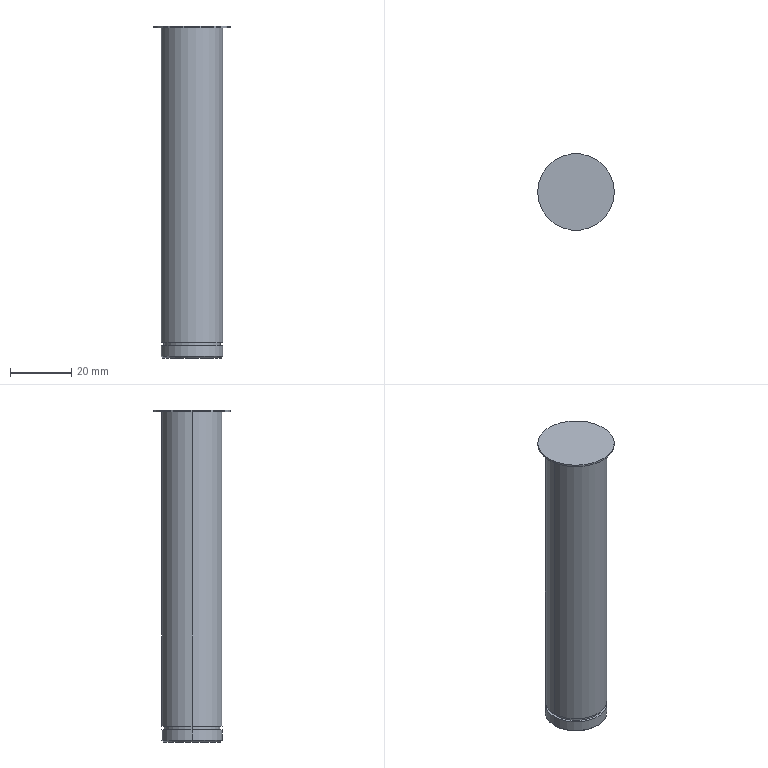Part | SolidWorks | features BaseBody 1 | 1 solid | 15 faces | box 25 x 25 x 108.34 mm | volume 34075 mm3 | cylinder 8 | plane 5 | cone 2 | commonest cylinder face diameters 20 x4 18.35 x2 25 x2
STEP:
#1=CARTESIAN_POINT('',(-9.5,0.,0.));
#2=VERTEX_POINT('',#1);
#3=CARTESIAN_POINT('',(9.5,0.,0.));
#4=VERTEX_POINT('',#3);
#5=CARTESIAN_POINT('',(0.,0.,0.));
#6=DIRECTION('',(0.,0.,1.));
#7=DIRECTION('',(-1.,0.,0.));
#8=AXIS2_PLACEMENT_3D('',#5,#6,#7);
#9=CIRCLE('',#8,9.5);
#10=EDGE_CURVE('',#2,#4,#9,.T.);
#11=ORIENTED_EDGE('',*,*,#10,.T.);
#12=CARTESIAN_POINT('',(10.,0.,0.5));
#13=VERTEX_POINT('',#12);
#14=CARTESIAN_POINT('',(9.75,0.,0.25));
#15=DIRECTION('',(0.7071,0.,0.7071));
#16=VECTOR('',#15,1000.);
#17=LINE('',#14,#16);
#18=EDGE_CURVE('',#4,#13,#17,.T.);
#19=ORIENTED_EDGE('',*,*,#18,.T.);
#20=CARTESIAN_POINT('',(-10.,0.,0.5));
#21=VERTEX_POINT('',#20);
#22=CARTESIAN_POINT('',(0.,0.,0.5));
#23=DIRECTION('',(0.,0.,-1.));
#24=DIRECTION('',(-1.,0.,0.));
#25=AXIS2_PLACEMENT_3D('',#22,#23,#24);
#26=CIRCLE('',#25,10.);
#27=EDGE_CURVE('',#13,#21,#26,.T.);
#28=ORIENTED_EDGE('',*,*,#27,.T.);
#29=CARTESIAN_POINT('',(-9.75,0.,0.25));
#30=DIRECTION('',(-0.7071,0.,0.7071));
#31=VECTOR('',#30,1000.);
#32=LINE('',#29,#31);
#33=EDGE_CURVE('',#2,#21,#32,.T.);
#34=ORIENTED_EDGE('',*,*,#33,.F.);
#35=EDGE_LOOP('',(#11,#19,#28,#34));
#36=FACE_OUTER_BOUND('',#35,.T.);
#37=CARTESIAN_POINT('',(0.,0.,0.25));
#38=DIRECTION('',(0.,0.,1.));
#39=DIRECTION('',(-1.,0.,0.));
#40=AXIS2_PLACEMENT_3D('',#37,#38,#39);
#41=CONICAL_SURFACE('',#40,9.75,0.7854);
#42=ADVANCED_FACE('',(#36),#41,.T.);
#43=CARTESIAN_POINT('',(-10.,0.,4.));
#44=VERTEX_POINT('',#43);
#45=CARTESIAN_POINT('',(10.,0.,4.));
#46=VERTEX_POINT('',#45);
#47=CARTESIAN_POINT('',(0.,0.,4.));
#48=DIRECTION('',(0.,0.,-1.));
#49=DIRECTION('',(-1.,0.,0.));
#50=AXIS2_PLACEMENT_3D('',#47,#48,#49);
#51=CIRCLE('',#50,10.);
#52=EDGE_CURVE('',#44,#46,#51,.T.);
#53=ORIENTED_EDGE('',*,*,#52,.T.);
#54=CARTESIAN_POINT('',(10.,0.,0.));
#55=DIRECTION('',(0.,0.,-1.));
#56=VECTOR('',#55,1000.);
#57=LINE('',#54,#56);
#58=EDGE_CURVE('',#46,#13,#57,.T.);
#59=ORIENTED_EDGE('',*,*,#58,.T.);
#60=CARTESIAN_POINT('',(0.,0.,0.5));
#61=DIRECTION('',(0.,0.,-1.));
#62=DIRECTION('',(-1.,0.,0.));
#63=AXIS2_PLACEMENT_3D('',#60,#61,#62);
#64=CIRCLE('',#63,10.);
#65=EDGE_CURVE('',#21,#13,#64,.T.);
#66=ORIENTED_EDGE('',*,*,#65,.F.);
#67=CARTESIAN_POINT('',(-10.,0.,0.));
#68=DIRECTION('',(0.,0.,-1.));
#69=VECTOR('',#68,1000.);
#70=LINE('',#67,#69);
#71=EDGE_CURVE('',#44,#21,#70,.T.);
#72=ORIENTED_EDGE('',*,*,#71,.F.);
#73=EDGE_LOOP('',(#53,#59,#66,#72));
#74=FACE_OUTER_BOUND('',#73,.T.);
#75=CARTESIAN_POINT('',(0.,0.,0.));
#76=DIRECTION('',(0.,0.,-1.));
#77=DIRECTION('',(-1.,0.,0.));
#78=AXIS2_PLACEMENT_3D('',#75,#76,#77);
#79=CYLINDRICAL_SURFACE('',#78,10.);
#80=ADVANCED_FACE('',(#74),#79,.T.);
#81=CARTESIAN_POINT('',(9.175,0.,5.2));
#82=VERTEX_POINT('',#81);
#83=CARTESIAN_POINT('',(-9.175,0.,5.2));
#84=VERTEX_POINT('',#83);
#85=CARTESIAN_POINT('',(0.,0.,5.2));
#86=DIRECTION('',(0.,0.,1.));
#87=DIRECTION('',(1.,0.,0.));
#88=AXIS2_PLACEMENT_3D('',#85,#86,#87);
#89=CIRCLE('',#88,9.175);
#90=EDGE_CURVE('',#82,#84,#89,.T.);
#91=ORIENTED_EDGE('',*,*,#90,.F.);
#92=CARTESIAN_POINT('',(9.175,0.,4.));
#93=VERTEX_POINT('',#92);
#94=CARTESIAN_POINT('',(9.175,0.,4.6));
#95=DIRECTION('',(0.,0.,-1.));
#96=VECTOR('',#95,1000.);
#97=LINE('',#94,#96);
#98=EDGE_CURVE('',#82,#93,#97,.T.);
#99=ORIENTED_EDGE('',*,*,#98,.T.);
#100=CARTESIAN_POINT('',(-9.175,0.,4.));
#101=VERTEX_POINT('',#100);
#102=CARTESIAN_POINT('',(0.,0.,4.));
#103=DIRECTION('',(0.,0.,1.));
#104=DIRECTION('',(1.,0.,0.));
#105=AXIS2_PLACEMENT_3D('',#102,#103,#104);
#106=CIRCLE('',#105,9.175);
#107=EDGE_CURVE('',#93,#101,#106,.T.);
#108=ORIENTED_EDGE('',*,*,#107,.T.);
#109=CARTESIAN_POINT('',(-9.175,0.,4.6));
#110=DIRECTION('',(0.,0.,-1.));
#111=VECTOR('',#110,1000.);
#112=LINE('',#109,#111);
#113=EDGE_CURVE('',#84,#101,#112,.T.);
#114=ORIENTED_EDGE('',*,*,#113,.F.);
#115=EDGE_LOOP('',(#91,#99,#108,#114));
#116=FACE_OUTER_BOUND('',#115,.T.);
#117=CARTESIAN_POINT('',(0.,0.,4.6));
#118=DIRECTION('',(0.,0.,-1.));
#119=DIRECTION('',(-1.,0.,0.));
#120=AXIS2_PLACEMENT_3D('',#117,#118,#119);
#121=CYLINDRICAL_SURFACE('',#120,9.175);
#122=ADVANCED_FACE('',(#116),#121,.T.);
#123=CARTESIAN_POINT('',(12.5,0.,107.74));
#124=VERTEX_POINT('',#123);
#125=CARTESIAN_POINT('',(-12.5,0.,107.74));
#126=VERTEX_POINT('',#125);
#127=CARTESIAN_POINT('',(0.,0.,107.74));
#128=DIRECTION('',(0.,0.,-1.));
#129=DIRECTION('',(-1.,0.,0.));
#130=AXIS2_PLACEMENT_3D('',#127,#128,#129);
#131=CIRCLE('',#130,12.5);
#132=EDGE_CURVE('',#124,#126,#131,.T.);
#133=ORIENTED_EDGE('',*,*,#132,.F.);
#134=CARTESIAN_POINT('',(12.5,0.,108.34));
#135=VERTEX_POINT('',#134);
#136=CARTESIAN_POINT('',(12.5,0.,108.34));
#137=DIRECTION('',(0.,0.,1.));
#138=VECTOR('',#137,1000.);
#139=LINE('',#136,#138);
#140=EDGE_CURVE('',#124,#135,#139,.T.);
#141=ORIENTED_EDGE('',*,*,#140,.T.);
#142=CARTESIAN_POINT('',(-12.5,0.,108.34));
#143=VERTEX_POINT('',#142);
#144=CARTESIAN_POINT('',(0.,0.,108.34));
#145=DIRECTION('',(0.,0.,-1.));
#146=DIRECTION('',(-1.,0.,0.));
#147=AXIS2_PLACEMENT_3D('',#144,#145,#146);
#148=CIRCLE('',#147,12.5);
#149=EDGE_CURVE('',#135,#143,#148,.T.);
#150=ORIENTED_EDGE('',*,*,#149,.T.);
#151=CARTESIAN_POINT('',(-12.5,0.,108.34));
#152=DIRECTION('',(0.,0.,1.));
#153=VECTOR('',#152,1000.);
#154=LINE('',#151,#153);
#155=EDGE_CURVE('',#126,#143,#154,.T.);
#156=ORIENTED_EDGE('',*,*,#155,.F.);
#157=EDGE_LOOP('',(#133,#141,#150,#156));
#158=FACE_OUTER_BOUND('',#157,.T.);
#159=CARTESIAN_POINT('',(0.,0.,108.34));
#160=DIRECTION('',(0.,0.,1.));
#161=DIRECTION('',(-1.,0.,0.));
#162=AXIS2_PLACEMENT_3D('',#159,#160,#161);
#163=CYLINDRICAL_SURFACE('',#162,12.5);
#164=ADVANCED_FACE('',(#158),#163,.T.);
#165=CARTESIAN_POINT('',(-10.,0.,107.74));
#166=VERTEX_POINT('',#165);
#167=CARTESIAN_POINT('',(10.,0.,107.74));
#168=VERTEX_POINT('',#167);
#169=CARTESIAN_POINT('',(0.,0.,107.74));
#170=DIRECTION('',(0.,0.,-1.));
#171=DIRECTION('',(-1.,0.,0.));
#172=AXIS2_PLACEMENT_3D('',#169,#170,#171);
#173=CIRCLE('',#172,10.);
#174=EDGE_CURVE('',#166,#168,#173,.T.);
#175=ORIENTED_EDGE('',*,*,#174,.T.);
#176=CARTESIAN_POINT('',(10.,0.,5.2));
#177=VERTEX_POINT('',#176);
#178=CARTESIAN_POINT('',(10.,0.,0.));
#179=DIRECTION('',(0.,0.,-1.));
#180=VECTOR('',#179,1000.);
#181=LINE('',#178,#180);
#182=EDGE_CURVE('',#168,#177,#181,.T.);
#183=ORIENTED_EDGE('',*,*,#182,.T.);
#184=CARTESIAN_POINT('',(-10.,0.,5.2));
#185=VERTEX_POINT('',#184);
#186=CARTESIAN_POINT('',(0.,0.,5.2));
#187=DIRECTION('',(0.,0.,1.));
#188=DIRECTION('',(-1.,0.,0.));
#189=AXIS2_PLACEMENT_3D('',#186,#187,#188);
#190=CIRCLE('',#189,10.);
#191=EDGE_CURVE('',#177,#185,#190,.T.);
#192=ORIENTED_EDGE('',*,*,#191,.T.);
#193=CARTESIAN_POINT('',(-10.,0.,0.));
#194=DIRECTION('',(0.,0.,-1.));
#195=VECTOR('',#194,1000.);
#196=LINE('',#193,#195);
#197=EDGE_CURVE('',#166,#185,#196,.T.);
#198=ORIENTED_EDGE('',*,*,#197,.F.);
#199=EDGE_LOOP('',(#175,#183,#192,#198));
#200=FACE_OUTER_BOUND('',#199,.T.);
#201=CARTESIAN_POINT('',(0.,0.,0.));
#202=DIRECTION('',(0.,0.,-1.));
#203=DIRECTION('',(-1.,0.,0.));
#204=AXIS2_PLACEMENT_3D('',#201,#202,#203);
#205=CYLINDRICAL_SURFACE('',#204,10.);
#206=ADVANCED_FACE('',(#200),#205,.T.);
#207=ORIENTED_EDGE('',*,*,#10,.F.);
#208=CARTESIAN_POINT('',(0.,0.,0.));
#209=DIRECTION('',(0.,0.,1.));
#210=DIRECTION('',(-1.,0.,0.));
#211=AXIS2_PLACEMENT_3D('',#208,#209,#210);
#212=CIRCLE('',#211,9.5);
#213=EDGE_CURVE('',#4,#2,#212,.T.);
#214=ORIENTED_EDGE('',*,*,#213,.F.);
#215=EDGE_LOOP('',(#207,#214));
#216=FACE_OUTER_BOUND('',#215,.T.);
#217=CARTESIAN_POINT('',(0.,0.,0.));
#218=DIRECTION('',(0.,0.,1.));
#219=DIRECTION('',(1.,0.,0.));
#220=AXIS2_PLACEMENT_3D('',#217,#218,#219);
#221=PLANE('',#220);
#222=ADVANCED_FACE('',(#216),#221,.F.);
#223=CARTESIAN_POINT('',(0.,0.,5.2));
#224=DIRECTION('',(0.,0.,1.));
#225=DIRECTION('',(1.,0.,0.));
#226=AXIS2_PLACEMENT_3D('',#223,#224,#225);
#227=CIRCLE('',#226,9.175);
#228=EDGE_CURVE('',#84,#82,#227,.T.);
#229=ORIENTED_EDGE('',*,*,#228,.T.);
#230=ORIENTED_EDGE('',*,*,#90,.T.);
#231=EDGE_LOOP('',(#229,#230));
#232=FACE_BOUND('',#231,.T.);
#233=CARTESIAN_POINT('',(0.,0.,5.2));
#234=DIRECTION('',(0.,0.,1.));
#235=DIRECTION('',(-1.,0.,0.));
#236=AXIS2_PLACEMENT_3D('',#233,#234,#235);
#237=CIRCLE('',#236,10.);
#238=EDGE_CURVE('',#185,#177,#237,.T.);
#239=ORIENTED_EDGE('',*,*,#238,.F.);
#240=ORIENTED_EDGE('',*,*,#191,.F.);
#241=EDGE_LOOP('',(#239,#240));
#242=FACE_OUTER_BOUND('',#241,.T.);
#243=CARTESIAN_POINT('',(-9.175,0.,5.2));
#244=DIRECTION('',(0.,0.,1.));
#245=DIRECTION('',(1.,0.,0.));
#246=AXIS2_PLACEMENT_3D('',#243,#244,#245);
#247=PLANE('',#246);
#248=ADVANCED_FACE('',(#232,#242),#247,.F.);
#249=CARTESIAN_POINT('',(0.,0.,4.));
#250=DIRECTION('',(0.,0.,1.));
#251=DIRECTION('',(1.,0.,0.));
#252=AXIS2_PLACEMENT_3D('',#249,#250,#251);
#253=CIRCLE('',#252,9.175);
#254=EDGE_CURVE('',#101,#93,#253,.T.);
#255=ORIENTED_EDGE('',*,*,#254,.F.);
#256=ORIENTED_EDGE('',*,*,#107,.F.);
#257=EDGE_LOOP('',(#255,#256));
#258=FACE_BOUND('',#257,.T.);
#259=ORIENTED_EDGE('',*,*,#52,.F.);
#260=CARTESIAN_POINT('',(0.,0.,4.));
#261=DIRECTION('',(0.,0.,-1.));
#262=DIRECTION('',(-1.,0.,0.));
#263=AXIS2_PLACEMENT_3D('',#260,#261,#262);
#264=CIRCLE('',#263,10.);
#265=EDGE_CURVE('',#46,#44,#264,.T.);
#266=ORIENTED_EDGE('',*,*,#265,.F.);
#267=EDGE_LOOP('',(#259,#266));
#268=FACE_OUTER_BOUND('',#267,.T.);
#269=CARTESIAN_POINT('',(-15.328,0.,4.));
#270=DIRECTION('',(0.,0.,-1.));
#271=DIRECTION('',(0.,-1.,0.));
#272=AXIS2_PLACEMENT_3D('',#269,#270,#271);
#273=PLANE('',#272);
#274=ADVANCED_FACE('',(#258,#268),#273,.F.);
#275=ORIENTED_EDGE('',*,*,#174,.F.);
#276=CARTESIAN_POINT('',(0.,0.,107.74));
#277=DIRECTION('',(0.,0.,-1.));
#278=DIRECTION('',(-1.,0.,0.));
#279=AXIS2_PLACEMENT_3D('',#276,#277,#278);
#280=CIRCLE('',#279,10.);
#281=EDGE_CURVE('',#168,#166,#280,.T.);
#282=ORIENTED_EDGE('',*,*,#281,.F.);
#283=EDGE_LOOP('',(#275,#282));
#284=FACE_BOUND('',#283,.T.);
#285=CARTESIAN_POINT('',(0.,0.,107.74));
#286=DIRECTION('',(0.,0.,-1.));
#287=DIRECTION('',(-1.,0.,0.));
#288=AXIS2_PLACEMENT_3D('',#285,#286,#287);
#289=CIRCLE('',#288,12.5);
#290=EDGE_CURVE('',#126,#124,#289,.T.);
#291=ORIENTED_EDGE('',*,*,#290,.T.);
#292=ORIENTED_EDGE('',*,*,#132,.T.);
#293=EDGE_LOOP('',(#291,#292));
#294=FACE_OUTER_BOUND('',#293,.T.);
#295=CARTESIAN_POINT('',(0.,0.,107.74));
#296=DIRECTION('',(0.,0.,1.));
#297=DIRECTION('',(1.,0.,0.));
#298=AXIS2_PLACEMENT_3D('',#295,#296,#297);
#299=PLANE('',#298);
#300=ADVANCED_FACE('',(#284,#294),#299,.F.);
#301=CARTESIAN_POINT('',(0.,0.,108.34));
#302=DIRECTION('',(0.,0.,-1.));
#303=DIRECTION('',(-1.,0.,0.));
#304=AXIS2_PLACEMENT_3D('',#301,#302,#303);
#305=CIRCLE('',#304,12.5);
#306=EDGE_CURVE('',#143,#135,#305,.T.);
#307=ORIENTED_EDGE('',*,*,#306,.F.);
#308=ORIENTED_EDGE('',*,*,#149,.F.);
#309=EDGE_LOOP('',(#307,#308));
#310=FACE_OUTER_BOUND('',#309,.T.);
#311=CARTESIAN_POINT('',(0.,0.,108.34));
#312=DIRECTION('',(0.,0.,1.));
#313=DIRECTION('',(1.,0.,0.));
#314=AXIS2_PLACEMENT_3D('',#311,#312,#313);
#315=PLANE('',#314);
#316=ADVANCED_FACE('',(#310),#315,.T.);
#317=ORIENTED_EDGE('',*,*,#182,.F.);
#318=ORIENTED_EDGE('',*,*,#281,.T.);
#319=ORIENTED_EDGE('',*,*,#197,.T.);
#320=ORIENTED_EDGE('',*,*,#238,.T.);
#321=EDGE_LOOP('',(#317,#318,#319,#320));
#322=FACE_OUTER_BOUND('',#321,.T.);
#323=CARTESIAN_POINT('',(0.,0.,0.));
#324=DIRECTION('',(0.,0.,-1.));
#325=DIRECTION('',(-1.,0.,0.));
#326=AXIS2_PLACEMENT_3D('',#323,#324,#325);
#327=CYLINDRICAL_SURFACE('',#326,10.);
#328=ADVANCED_FACE('',(#322),#327,.T.);
#329=ORIENTED_EDGE('',*,*,#140,.F.);
#330=ORIENTED_EDGE('',*,*,#290,.F.);
#331=ORIENTED_EDGE('',*,*,#155,.T.);
#332=ORIENTED_EDGE('',*,*,#306,.T.);
#333=EDGE_LOOP('',(#329,#330,#331,#332));
#334=FACE_OUTER_BOUND('',#333,.T.);
#335=CARTESIAN_POINT('',(0.,0.,108.34));
#336=DIRECTION('',(0.,0.,1.));
#337=DIRECTION('',(-1.,0.,0.));
#338=AXIS2_PLACEMENT_3D('',#335,#336,#337);
#339=CYLINDRICAL_SURFACE('',#338,12.5);
#340=ADVANCED_FACE('',(#334),#339,.T.);
#341=ORIENTED_EDGE('',*,*,#98,.F.);
#342=ORIENTED_EDGE('',*,*,#228,.F.);
#343=ORIENTED_EDGE('',*,*,#113,.T.);
#344=ORIENTED_EDGE('',*,*,#254,.T.);
#345=EDGE_LOOP('',(#341,#342,#343,#344));
#346=FACE_OUTER_BOUND('',#345,.T.);
#347=CARTESIAN_POINT('',(0.,0.,4.6));
#348=DIRECTION('',(0.,0.,-1.));
#349=DIRECTION('',(-1.,0.,0.));
#350=AXIS2_PLACEMENT_3D('',#347,#348,#349);
#351=CYLINDRICAL_SURFACE('',#350,9.175);
#352=ADVANCED_FACE('',(#346),#351,.T.);
#353=ORIENTED_EDGE('',*,*,#58,.F.);
#354=ORIENTED_EDGE('',*,*,#265,.T.);
#355=ORIENTED_EDGE('',*,*,#71,.T.);
#356=ORIENTED_EDGE('',*,*,#27,.F.);
#357=EDGE_LOOP('',(#353,#354,#355,#356));
#358=FACE_OUTER_BOUND('',#357,.T.);
#359=CARTESIAN_POINT('',(0.,0.,0.));
#360=DIRECTION('',(0.,0.,-1.));
#361=DIRECTION('',(-1.,0.,0.));
#362=AXIS2_PLACEMENT_3D('',#359,#360,#361);
#363=CYLINDRICAL_SURFACE('',#362,10.);
#364=ADVANCED_FACE('',(#358),#363,.T.);
#365=ORIENTED_EDGE('',*,*,#18,.F.);
#366=ORIENTED_EDGE('',*,*,#213,.T.);
#367=ORIENTED_EDGE('',*,*,#33,.T.);
#368=ORIENTED_EDGE('',*,*,#65,.T.);
#369=EDGE_LOOP('',(#365,#366,#367,#368));
#370=FACE_OUTER_BOUND('',#369,.T.);
#371=CARTESIAN_POINT('',(0.,0.,0.25));
#372=DIRECTION('',(0.,0.,1.));
#373=DIRECTION('',(-1.,0.,0.));
#374=AXIS2_PLACEMENT_3D('',#371,#372,#373);
#375=CONICAL_SURFACE('',#374,9.75,0.7854);
#376=ADVANCED_FACE('',(#370),#375,.T.);
#377=CLOSED_SHELL('',(#42,#80,#122,#164,#206,#222,#248,#274,#300,#316,#328,#340,#352,#364,#376));
#378=MANIFOLD_SOLID_BREP('',#377);
#379=CARTESIAN_POINT('',(0.,0.,0.));
#380=DIRECTION('',(0.,0.,1.));
#381=DIRECTION('',(1.,0.,0.));
#382=AXIS2_PLACEMENT_3D('',#379,#380,#381);
#383=(LENGTH_UNIT()NAMED_UNIT(*)SI_UNIT(.MILLI.,.METRE.));
#384=UNCERTAINTY_MEASURE_WITH_UNIT(LENGTH_MEASURE(0.00001),#383,'','');
#385=(NAMED_UNIT(*)PLANE_ANGLE_UNIT()SI_UNIT($,.RADIAN.));
#386=(NAMED_UNIT(*)SI_UNIT($,.STERADIAN.)SOLID_ANGLE_UNIT());
#387=(GEOMETRIC_REPRESENTATION_CONTEXT(3)GLOBAL_UNCERTAINTY_ASSIGNED_CONTEXT((#384))GLOBAL_UNIT_ASSIGNED_CONTEXT((#383,#385,#386))REPRESENTATION_CONTEXT('',''));
#388=ADVANCED_BREP_SHAPE_REPRESENTATION('',(#378,#382),#387);